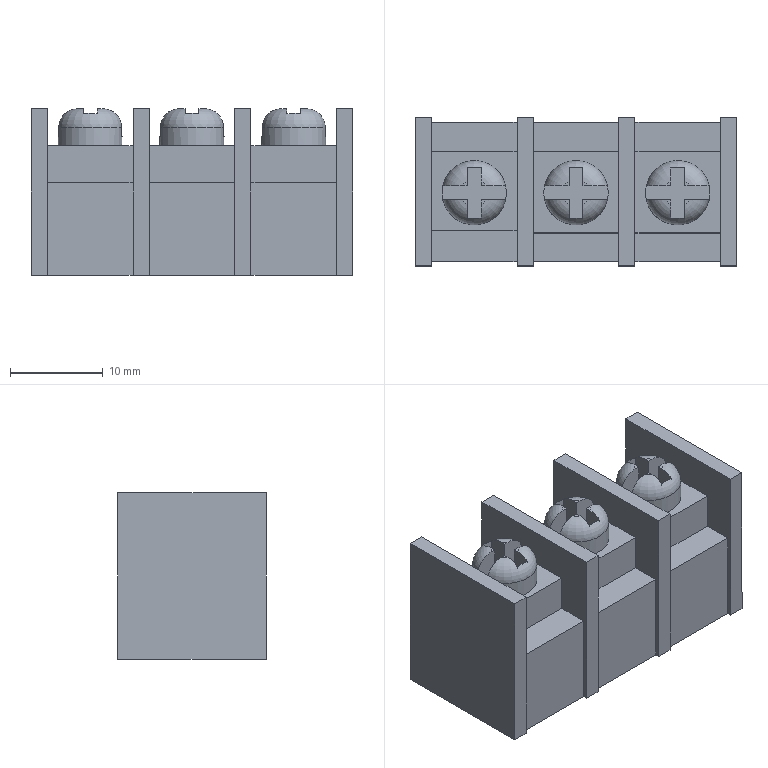Part | NX | features BREP 1 | 1 solid | 96 faces | box 34.75 x 16 x 18 mm | volume 7444 mm3 | plane 87 | torus 6 | cylinder 3 | commonest cylinder face diameters 6.956 x3